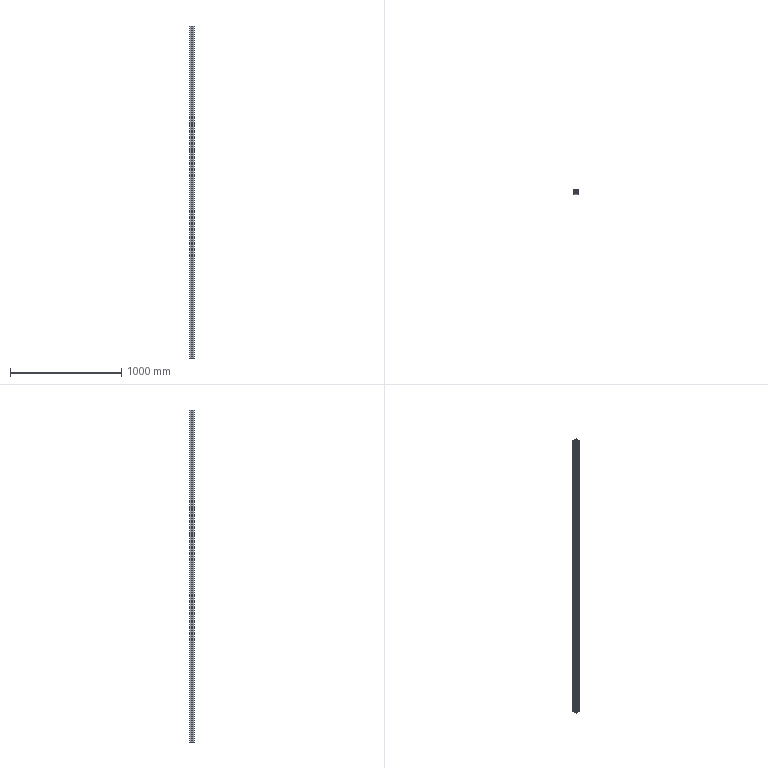Part | STEP file | 40_40_4640_1-2 | 1 solid | 64 faces | box 40 x 40 x 2989 mm | volume 1568656 mm3 | plane 62 | cylinder 2 | commonest cylinder face diameters 6.8 x2